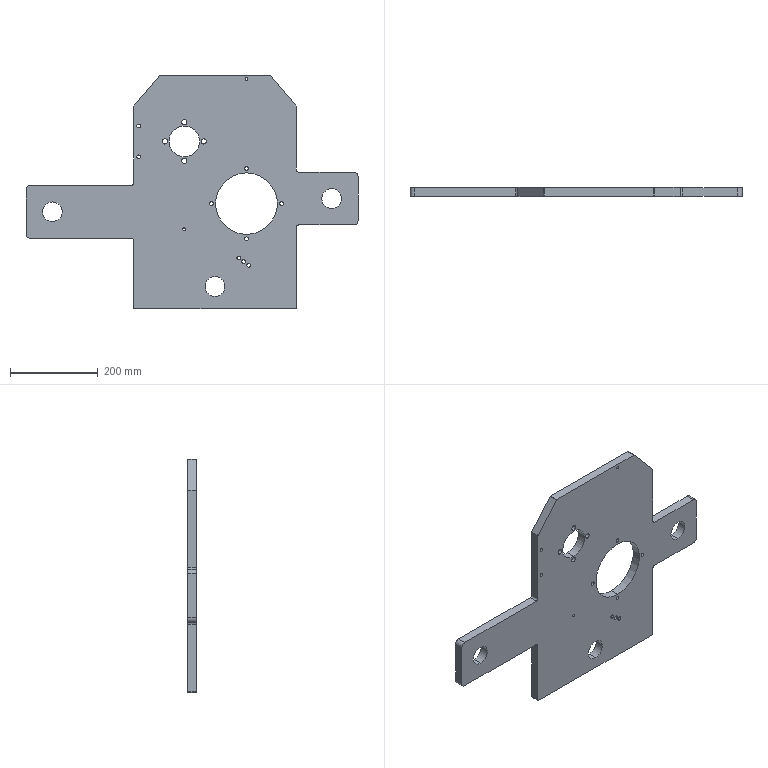Part | SolidWorks | features BaseBody 1 | 1 solid | 70 faces | box 755 x 20 x 530 mm | volume 4259685 mm3 | cylinder 54 | plane 16 | commonest cylinder face diameters 8.5 x18 12 x8 4 x6 45 x6 6.8 x4 10 x4